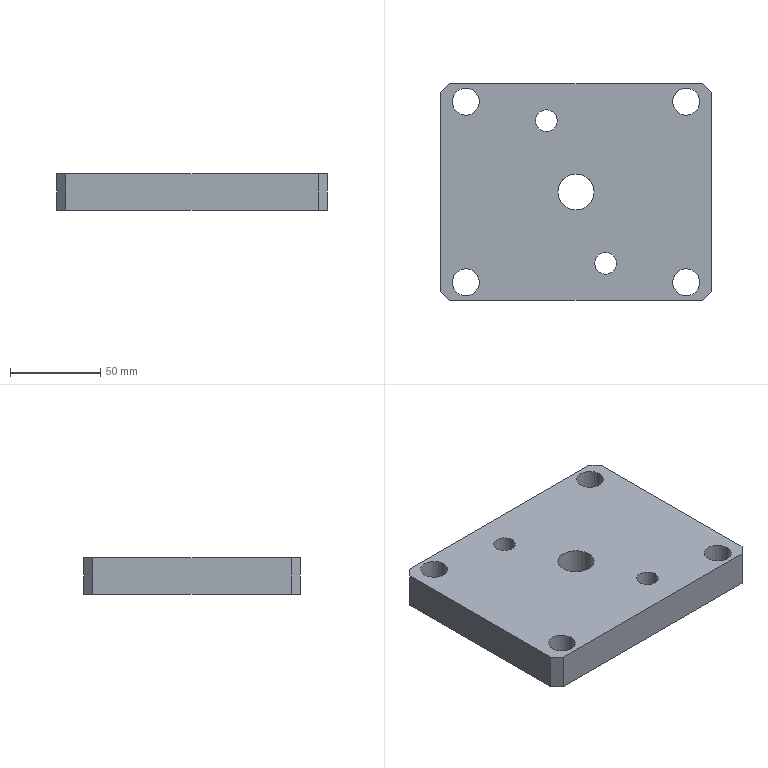Part | SolidWorks | features Cut 2, Extrusion 1, ICE 1 | 1 solid | 24 faces | box 150 x 120 x 20 mm | volume 334056 mm3 | cylinder 14 | plane 10 | commonest cylinder face diameters 15 x8 12 x4 20 x2
STEP:
#1=CARTESIAN_POINT('',(10.379,-39.542,20.));
#2=VERTEX_POINT('',#1);
#3=CARTESIAN_POINT('',(22.379,-39.542,20.));
#4=VERTEX_POINT('',#3);
#5=CARTESIAN_POINT('',(16.379,-39.542,20.));
#6=DIRECTION('',(0.,0.,1.));
#7=DIRECTION('',(-1.,0.,0.));
#8=AXIS2_PLACEMENT_3D('',#5,#6,#7);
#9=CIRCLE('',#8,6.);
#10=EDGE_CURVE('',#2,#4,#9,.T.);
#11=ORIENTED_EDGE('',*,*,#10,.T.);
#12=CARTESIAN_POINT('',(22.379,-39.542,0.));
#13=VERTEX_POINT('',#12);
#14=CARTESIAN_POINT('',(22.379,-39.542,36.971));
#15=DIRECTION('',(0.,0.,-1.));
#16=VECTOR('',#15,1000.);
#17=LINE('',#14,#16);
#18=EDGE_CURVE('',#4,#13,#17,.T.);
#19=ORIENTED_EDGE('',*,*,#18,.T.);
#20=CARTESIAN_POINT('',(10.379,-39.542,0.));
#21=VERTEX_POINT('',#20);
#22=CARTESIAN_POINT('',(16.379,-39.542,0.));
#23=DIRECTION('',(0.,0.,-1.));
#24=DIRECTION('',(-1.,0.,0.));
#25=AXIS2_PLACEMENT_3D('',#22,#23,#24);
#26=CIRCLE('',#25,6.);
#27=EDGE_CURVE('',#13,#21,#26,.T.);
#28=ORIENTED_EDGE('',*,*,#27,.T.);
#29=CARTESIAN_POINT('',(10.379,-39.542,36.971));
#30=DIRECTION('',(0.,0.,-1.));
#31=VECTOR('',#30,1000.);
#32=LINE('',#29,#31);
#33=EDGE_CURVE('',#2,#21,#32,.T.);
#34=ORIENTED_EDGE('',*,*,#33,.F.);
#35=EDGE_LOOP('',(#11,#19,#28,#34));
#36=FACE_OUTER_BOUND('',#35,.T.);
#37=CARTESIAN_POINT('',(16.379,-39.542,36.971));
#38=DIRECTION('',(0.,0.,-1.));
#39=DIRECTION('',(-1.,0.,0.));
#40=AXIS2_PLACEMENT_3D('',#37,#38,#39);
#41=CYLINDRICAL_SURFACE('',#40,6.);
#42=ADVANCED_FACE('',(#36),#41,.F.);
#43=CARTESIAN_POINT('',(-22.379,39.542,20.));
#44=VERTEX_POINT('',#43);
#45=CARTESIAN_POINT('',(-10.379,39.542,20.));
#46=VERTEX_POINT('',#45);
#47=CARTESIAN_POINT('',(-16.379,39.542,20.));
#48=DIRECTION('',(0.,0.,1.));
#49=DIRECTION('',(-1.,0.,0.));
#50=AXIS2_PLACEMENT_3D('',#47,#48,#49);
#51=CIRCLE('',#50,6.);
#52=EDGE_CURVE('',#44,#46,#51,.T.);
#53=ORIENTED_EDGE('',*,*,#52,.T.);
#54=CARTESIAN_POINT('',(-10.379,39.542,0.));
#55=VERTEX_POINT('',#54);
#56=CARTESIAN_POINT('',(-10.379,39.542,36.971));
#57=DIRECTION('',(0.,0.,-1.));
#58=VECTOR('',#57,1000.);
#59=LINE('',#56,#58);
#60=EDGE_CURVE('',#46,#55,#59,.T.);
#61=ORIENTED_EDGE('',*,*,#60,.T.);
#62=CARTESIAN_POINT('',(-22.379,39.542,0.));
#63=VERTEX_POINT('',#62);
#64=CARTESIAN_POINT('',(-16.379,39.542,0.));
#65=DIRECTION('',(0.,0.,-1.));
#66=DIRECTION('',(-1.,0.,0.));
#67=AXIS2_PLACEMENT_3D('',#64,#65,#66);
#68=CIRCLE('',#67,6.);
#69=EDGE_CURVE('',#55,#63,#68,.T.);
#70=ORIENTED_EDGE('',*,*,#69,.T.);
#71=CARTESIAN_POINT('',(-22.379,39.542,36.971));
#72=DIRECTION('',(0.,0.,-1.));
#73=VECTOR('',#72,1000.);
#74=LINE('',#71,#73);
#75=EDGE_CURVE('',#44,#63,#74,.T.);
#76=ORIENTED_EDGE('',*,*,#75,.F.);
#77=EDGE_LOOP('',(#53,#61,#70,#76));
#78=FACE_OUTER_BOUND('',#77,.T.);
#79=CARTESIAN_POINT('',(-16.379,39.542,36.971));
#80=DIRECTION('',(0.,0.,-1.));
#81=DIRECTION('',(-1.,0.,0.));
#82=AXIS2_PLACEMENT_3D('',#79,#80,#81);
#83=CYLINDRICAL_SURFACE('',#82,6.);
#84=ADVANCED_FACE('',(#78),#83,.F.);
#85=CARTESIAN_POINT('',(10.,0.,20.));
#86=VERTEX_POINT('',#85);
#87=CARTESIAN_POINT('',(-10.,0.,20.));
#88=VERTEX_POINT('',#87);
#89=CARTESIAN_POINT('',(0.,0.,20.));
#90=DIRECTION('',(0.,0.,-1.));
#91=DIRECTION('',(-1.,0.,0.));
#92=AXIS2_PLACEMENT_3D('',#89,#90,#91);
#93=CIRCLE('',#92,10.);
#94=EDGE_CURVE('',#86,#88,#93,.T.);
#95=ORIENTED_EDGE('',*,*,#94,.F.);
#96=CARTESIAN_POINT('',(10.,0.,0.));
#97=VERTEX_POINT('',#96);
#98=CARTESIAN_POINT('',(10.,0.,59.));
#99=DIRECTION('',(0.,0.,-1.));
#100=VECTOR('',#99,1000.);
#101=LINE('',#98,#100);
#102=EDGE_CURVE('',#86,#97,#101,.T.);
#103=ORIENTED_EDGE('',*,*,#102,.T.);
#104=CARTESIAN_POINT('',(-10.,0.,0.));
#105=VERTEX_POINT('',#104);
#106=CARTESIAN_POINT('',(0.,0.,0.));
#107=DIRECTION('',(0.,0.,-1.));
#108=DIRECTION('',(-1.,0.,0.));
#109=AXIS2_PLACEMENT_3D('',#106,#107,#108);
#110=CIRCLE('',#109,10.);
#111=EDGE_CURVE('',#97,#105,#110,.T.);
#112=ORIENTED_EDGE('',*,*,#111,.T.);
#113=CARTESIAN_POINT('',(-10.,0.,59.));
#114=DIRECTION('',(0.,0.,-1.));
#115=VECTOR('',#114,1000.);
#116=LINE('',#113,#115);
#117=EDGE_CURVE('',#88,#105,#116,.T.);
#118=ORIENTED_EDGE('',*,*,#117,.F.);
#119=EDGE_LOOP('',(#95,#103,#112,#118));
#120=FACE_OUTER_BOUND('',#119,.T.);
#121=CARTESIAN_POINT('',(0.,0.,59.));
#122=DIRECTION('',(0.,0.,-1.));
#123=DIRECTION('',(-1.,0.,0.));
#124=AXIS2_PLACEMENT_3D('',#121,#122,#123);
#125=CYLINDRICAL_SURFACE('',#124,10.);
#126=ADVANCED_FACE('',(#120),#125,.F.);
#127=CARTESIAN_POINT('',(-53.5,50.,20.));
#128=VERTEX_POINT('',#127);
#129=CARTESIAN_POINT('',(-68.5,50.,20.));
#130=VERTEX_POINT('',#129);
#131=CARTESIAN_POINT('',(-61.,50.,20.));
#132=DIRECTION('',(0.,0.,-1.));
#133=DIRECTION('',(1.,0.,0.));
#134=AXIS2_PLACEMENT_3D('',#131,#132,#133);
#135=CIRCLE('',#134,7.5);
#136=EDGE_CURVE('',#128,#130,#135,.T.);
#137=ORIENTED_EDGE('',*,*,#136,.F.);
#138=CARTESIAN_POINT('',(-53.5,50.,0.));
#139=VERTEX_POINT('',#138);
#140=CARTESIAN_POINT('',(-53.5,50.,20.));
#141=DIRECTION('',(0.,0.,-1.));
#142=VECTOR('',#141,1000.);
#143=LINE('',#140,#142);
#144=EDGE_CURVE('',#128,#139,#143,.T.);
#145=ORIENTED_EDGE('',*,*,#144,.T.);
#146=CARTESIAN_POINT('',(-68.5,50.,0.));
#147=VERTEX_POINT('',#146);
#148=CARTESIAN_POINT('',(-61.,50.,0.));
#149=DIRECTION('',(0.,0.,-1.));
#150=DIRECTION('',(-1.,0.,0.));
#151=AXIS2_PLACEMENT_3D('',#148,#149,#150);
#152=CIRCLE('',#151,7.5);
#153=EDGE_CURVE('',#139,#147,#152,.T.);
#154=ORIENTED_EDGE('',*,*,#153,.T.);
#155=CARTESIAN_POINT('',(-68.5,50.,20.));
#156=DIRECTION('',(0.,0.,-1.));
#157=VECTOR('',#156,1000.);
#158=LINE('',#155,#157);
#159=EDGE_CURVE('',#130,#147,#158,.T.);
#160=ORIENTED_EDGE('',*,*,#159,.F.);
#161=EDGE_LOOP('',(#137,#145,#154,#160));
#162=FACE_OUTER_BOUND('',#161,.T.);
#163=CARTESIAN_POINT('',(-61.,50.,20.));
#164=DIRECTION('',(0.,0.,-1.));
#165=DIRECTION('',(-1.,0.,0.));
#166=AXIS2_PLACEMENT_3D('',#163,#164,#165);
#167=CYLINDRICAL_SURFACE('',#166,7.5);
#168=ADVANCED_FACE('',(#162),#167,.F.);
#169=CARTESIAN_POINT('',(68.5,-50.,20.));
#170=VERTEX_POINT('',#169);
#171=CARTESIAN_POINT('',(53.5,-50.,20.));
#172=VERTEX_POINT('',#171);
#173=CARTESIAN_POINT('',(61.,-50.,20.));
#174=DIRECTION('',(0.,0.,-1.));
#175=DIRECTION('',(1.,0.,0.));
#176=AXIS2_PLACEMENT_3D('',#173,#174,#175);
#177=CIRCLE('',#176,7.5);
#178=EDGE_CURVE('',#170,#172,#177,.T.);
#179=ORIENTED_EDGE('',*,*,#178,.F.);
#180=CARTESIAN_POINT('',(68.5,-50.,0.));
#181=VERTEX_POINT('',#180);
#182=CARTESIAN_POINT('',(68.5,-50.,20.));
#183=DIRECTION('',(0.,0.,-1.));
#184=VECTOR('',#183,1000.);
#185=LINE('',#182,#184);
#186=EDGE_CURVE('',#170,#181,#185,.T.);
#187=ORIENTED_EDGE('',*,*,#186,.T.);
#188=CARTESIAN_POINT('',(53.5,-50.,0.));
#189=VERTEX_POINT('',#188);
#190=CARTESIAN_POINT('',(61.,-50.,0.));
#191=DIRECTION('',(0.,0.,-1.));
#192=DIRECTION('',(-1.,0.,0.));
#193=AXIS2_PLACEMENT_3D('',#190,#191,#192);
#194=CIRCLE('',#193,7.5);
#195=EDGE_CURVE('',#181,#189,#194,.T.);
#196=ORIENTED_EDGE('',*,*,#195,.T.);
#197=CARTESIAN_POINT('',(53.5,-50.,20.));
#198=DIRECTION('',(0.,0.,-1.));
#199=VECTOR('',#198,1000.);
#200=LINE('',#197,#199);
#201=EDGE_CURVE('',#172,#189,#200,.T.);
#202=ORIENTED_EDGE('',*,*,#201,.F.);
#203=EDGE_LOOP('',(#179,#187,#196,#202));
#204=FACE_OUTER_BOUND('',#203,.T.);
#205=CARTESIAN_POINT('',(61.,-50.,20.));
#206=DIRECTION('',(0.,0.,-1.));
#207=DIRECTION('',(-1.,0.,0.));
#208=AXIS2_PLACEMENT_3D('',#205,#206,#207);
#209=CYLINDRICAL_SURFACE('',#208,7.5);
#210=ADVANCED_FACE('',(#204),#209,.F.);
#211=CARTESIAN_POINT('',(68.5,50.,20.));
#212=VERTEX_POINT('',#211);
#213=CARTESIAN_POINT('',(53.5,50.,20.));
#214=VERTEX_POINT('',#213);
#215=CARTESIAN_POINT('',(61.,50.,20.));
#216=DIRECTION('',(0.,0.,-1.));
#217=DIRECTION('',(-1.,0.,0.));
#218=AXIS2_PLACEMENT_3D('',#215,#216,#217);
#219=CIRCLE('',#218,7.5);
#220=EDGE_CURVE('',#212,#214,#219,.T.);
#221=ORIENTED_EDGE('',*,*,#220,.F.);
#222=CARTESIAN_POINT('',(68.5,50.,0.));
#223=VERTEX_POINT('',#222);
#224=CARTESIAN_POINT('',(68.5,50.,20.));
#225=DIRECTION('',(0.,0.,-1.));
#226=VECTOR('',#225,1000.);
#227=LINE('',#224,#226);
#228=EDGE_CURVE('',#212,#223,#227,.T.);
#229=ORIENTED_EDGE('',*,*,#228,.T.);
#230=CARTESIAN_POINT('',(53.5,50.,0.));
#231=VERTEX_POINT('',#230);
#232=CARTESIAN_POINT('',(61.,50.,0.));
#233=DIRECTION('',(0.,0.,-1.));
#234=DIRECTION('',(-1.,0.,0.));
#235=AXIS2_PLACEMENT_3D('',#232,#233,#234);
#236=CIRCLE('',#235,7.5);
#237=EDGE_CURVE('',#223,#231,#236,.T.);
#238=ORIENTED_EDGE('',*,*,#237,.T.);
#239=CARTESIAN_POINT('',(53.5,50.,20.));
#240=DIRECTION('',(0.,0.,-1.));
#241=VECTOR('',#240,1000.);
#242=LINE('',#239,#241);
#243=EDGE_CURVE('',#214,#231,#242,.T.);
#244=ORIENTED_EDGE('',*,*,#243,.F.);
#245=EDGE_LOOP('',(#221,#229,#238,#244));
#246=FACE_OUTER_BOUND('',#245,.T.);
#247=CARTESIAN_POINT('',(61.,50.,20.));
#248=DIRECTION('',(0.,0.,-1.));
#249=DIRECTION('',(-1.,0.,0.));
#250=AXIS2_PLACEMENT_3D('',#247,#248,#249);
#251=CYLINDRICAL_SURFACE('',#250,7.5);
#252=ADVANCED_FACE('',(#246),#251,.F.);
#253=CARTESIAN_POINT('',(-53.5,-50.,20.));
#254=VERTEX_POINT('',#253);
#255=CARTESIAN_POINT('',(-68.5,-50.,20.));
#256=VERTEX_POINT('',#255);
#257=CARTESIAN_POINT('',(-61.,-50.,20.));
#258=DIRECTION('',(0.,0.,-1.));
#259=DIRECTION('',(-1.,0.,0.));
#260=AXIS2_PLACEMENT_3D('',#257,#258,#259);
#261=CIRCLE('',#260,7.5);
#262=EDGE_CURVE('',#254,#256,#261,.T.);
#263=ORIENTED_EDGE('',*,*,#262,.F.);
#264=CARTESIAN_POINT('',(-53.5,-50.,0.));
#265=VERTEX_POINT('',#264);
#266=CARTESIAN_POINT('',(-53.5,-50.,20.));
#267=DIRECTION('',(0.,0.,-1.));
#268=VECTOR('',#267,1000.);
#269=LINE('',#266,#268);
#270=EDGE_CURVE('',#254,#265,#269,.T.);
#271=ORIENTED_EDGE('',*,*,#270,.T.);
#272=CARTESIAN_POINT('',(-68.5,-50.,0.));
#273=VERTEX_POINT('',#272);
#274=CARTESIAN_POINT('',(-61.,-50.,0.));
#275=DIRECTION('',(0.,0.,-1.));
#276=DIRECTION('',(-1.,0.,0.));
#277=AXIS2_PLACEMENT_3D('',#274,#275,#276);
#278=CIRCLE('',#277,7.5);
#279=EDGE_CURVE('',#265,#273,#278,.T.);
#280=ORIENTED_EDGE('',*,*,#279,.T.);
#281=CARTESIAN_POINT('',(-68.5,-50.,20.));
#282=DIRECTION('',(0.,0.,-1.));
#283=VECTOR('',#282,1000.);
#284=LINE('',#281,#283);
#285=EDGE_CURVE('',#256,#273,#284,.T.);
#286=ORIENTED_EDGE('',*,*,#285,.F.);
#287=EDGE_LOOP('',(#263,#271,#280,#286));
#288=FACE_OUTER_BOUND('',#287,.T.);
#289=CARTESIAN_POINT('',(-61.,-50.,20.));
#290=DIRECTION('',(0.,0.,-1.));
#291=DIRECTION('',(-1.,0.,0.));
#292=AXIS2_PLACEMENT_3D('',#289,#290,#291);
#293=CYLINDRICAL_SURFACE('',#292,7.5);
#294=ADVANCED_FACE('',(#288),#293,.F.);
#295=CARTESIAN_POINT('',(-70.,-60.,0.));
#296=VERTEX_POINT('',#295);
#297=CARTESIAN_POINT('',(70.,-60.,0.));
#298=VERTEX_POINT('',#297);
#299=CARTESIAN_POINT('',(70.,-60.,0.));
#300=DIRECTION('',(1.,0.,0.));
#301=VECTOR('',#300,1000.);
#302=LINE('',#299,#301);
#303=EDGE_CURVE('',#296,#298,#302,.T.);
#304=ORIENTED_EDGE('',*,*,#303,.T.);
#305=CARTESIAN_POINT('',(70.,-60.,20.));
#306=VERTEX_POINT('',#305);
#307=CARTESIAN_POINT('',(70.,-60.,20.));
#308=DIRECTION('',(0.,0.,-1.));
#309=VECTOR('',#308,1000.);
#310=LINE('',#307,#309);
#311=EDGE_CURVE('',#306,#298,#310,.T.);
#312=ORIENTED_EDGE('',*,*,#311,.F.);
#313=CARTESIAN_POINT('',(-70.,-60.,20.));
#314=VERTEX_POINT('',#313);
#315=CARTESIAN_POINT('',(70.,-60.,20.));
#316=DIRECTION('',(1.,0.,0.));
#317=VECTOR('',#316,1000.);
#318=LINE('',#315,#317);
#319=EDGE_CURVE('',#314,#306,#318,.T.);
#320=ORIENTED_EDGE('',*,*,#319,.F.);
#321=CARTESIAN_POINT('',(-70.,-60.,20.));
#322=DIRECTION('',(0.,0.,-1.));
#323=VECTOR('',#322,1000.);
#324=LINE('',#321,#323);
#325=EDGE_CURVE('',#314,#296,#324,.T.);
#326=ORIENTED_EDGE('',*,*,#325,.T.);
#327=EDGE_LOOP('',(#304,#312,#320,#326));
#328=FACE_OUTER_BOUND('',#327,.T.);
#329=CARTESIAN_POINT('',(70.,-60.,20.));
#330=DIRECTION('',(0.,1.,0.));
#331=DIRECTION('',(-1.,0.,0.));
#332=AXIS2_PLACEMENT_3D('',#329,#330,#331);
#333=PLANE('',#332);
#334=ADVANCED_FACE('',(#328),#333,.F.);
#335=CARTESIAN_POINT('',(75.,-55.,0.));
#336=VERTEX_POINT('',#335);
#337=CARTESIAN_POINT('',(75.,-55.,0.));
#338=DIRECTION('',(0.7071,0.7071,0.));
#339=VECTOR('',#338,1000.);
#340=LINE('',#337,#339);
#341=EDGE_CURVE('',#298,#336,#340,.T.);
#342=ORIENTED_EDGE('',*,*,#341,.T.);
#343=CARTESIAN_POINT('',(75.,-55.,20.));
#344=VERTEX_POINT('',#343);
#345=CARTESIAN_POINT('',(75.,-55.,20.));
#346=DIRECTION('',(0.,0.,-1.));
#347=VECTOR('',#346,1000.);
#348=LINE('',#345,#347);
#349=EDGE_CURVE('',#344,#336,#348,.T.);
#350=ORIENTED_EDGE('',*,*,#349,.F.);
#351=CARTESIAN_POINT('',(75.,-55.,20.));
#352=DIRECTION('',(0.7071,0.7071,0.));
#353=VECTOR('',#352,1000.);
#354=LINE('',#351,#353);
#355=EDGE_CURVE('',#306,#344,#354,.T.);
#356=ORIENTED_EDGE('',*,*,#355,.F.);
#357=ORIENTED_EDGE('',*,*,#311,.T.);
#358=EDGE_LOOP('',(#342,#350,#356,#357));
#359=FACE_OUTER_BOUND('',#358,.T.);
#360=CARTESIAN_POINT('',(75.,-55.,20.));
#361=DIRECTION('',(-0.7071,0.7071,0.));
#362=DIRECTION('',(-0.7071,-0.7071,0.));
#363=AXIS2_PLACEMENT_3D('',#360,#361,#362);
#364=PLANE('',#363);
#365=ADVANCED_FACE('',(#359),#364,.F.);
#366=CARTESIAN_POINT('',(75.,55.,0.));
#367=VERTEX_POINT('',#366);
#368=CARTESIAN_POINT('',(75.,-55.,0.));
#369=DIRECTION('',(0.,1.,0.));
#370=VECTOR('',#369,1000.);
#371=LINE('',#368,#370);
#372=EDGE_CURVE('',#336,#367,#371,.T.);
#373=ORIENTED_EDGE('',*,*,#372,.T.);
#374=CARTESIAN_POINT('',(75.,55.,20.));
#375=VERTEX_POINT('',#374);
#376=CARTESIAN_POINT('',(75.,55.,20.));
#377=DIRECTION('',(0.,0.,-1.));
#378=VECTOR('',#377,1000.);
#379=LINE('',#376,#378);
#380=EDGE_CURVE('',#375,#367,#379,.T.);
#381=ORIENTED_EDGE('',*,*,#380,.F.);
#382=CARTESIAN_POINT('',(75.,-55.,20.));
#383=DIRECTION('',(0.,1.,0.));
#384=VECTOR('',#383,1000.);
#385=LINE('',#382,#384);
#386=EDGE_CURVE('',#344,#375,#385,.T.);
#387=ORIENTED_EDGE('',*,*,#386,.F.);
#388=ORIENTED_EDGE('',*,*,#349,.T.);
#389=EDGE_LOOP('',(#373,#381,#387,#388));
#390=FACE_OUTER_BOUND('',#389,.T.);
#391=CARTESIAN_POINT('',(75.,-55.,20.));
#392=DIRECTION('',(-1.,0.,0.));
#393=DIRECTION('',(0.,0.,1.));
#394=AXIS2_PLACEMENT_3D('',#391,#392,#393);
#395=PLANE('',#394);
#396=ADVANCED_FACE('',(#390),#395,.F.);
#397=CARTESIAN_POINT('',(70.,60.,0.));
#398=VERTEX_POINT('',#397);
#399=CARTESIAN_POINT('',(75.,55.,0.));
#400=DIRECTION('',(-0.7071,0.7071,0.));
#401=VECTOR('',#400,1000.);
#402=LINE('',#399,#401);
#403=EDGE_CURVE('',#367,#398,#402,.T.);
#404=ORIENTED_EDGE('',*,*,#403,.T.);
#405=CARTESIAN_POINT('',(70.,60.,20.));
#406=VERTEX_POINT('',#405);
#407=CARTESIAN_POINT('',(70.,60.,20.));
#408=DIRECTION('',(0.,0.,-1.));
#409=VECTOR('',#408,1000.);
#410=LINE('',#407,#409);
#411=EDGE_CURVE('',#406,#398,#410,.T.);
#412=ORIENTED_EDGE('',*,*,#411,.F.);
#413=CARTESIAN_POINT('',(75.,55.,20.));
#414=DIRECTION('',(-0.7071,0.7071,0.));
#415=VECTOR('',#414,1000.);
#416=LINE('',#413,#415);
#417=EDGE_CURVE('',#375,#406,#416,.T.);
#418=ORIENTED_EDGE('',*,*,#417,.F.);
#419=ORIENTED_EDGE('',*,*,#380,.T.);
#420=EDGE_LOOP('',(#404,#412,#418,#419));
#421=FACE_OUTER_BOUND('',#420,.T.);
#422=CARTESIAN_POINT('',(75.,55.,20.));
#423=DIRECTION('',(-0.7071,-0.7071,0.));
#424=DIRECTION('',(0.7071,-0.7071,0.));
#425=AXIS2_PLACEMENT_3D('',#422,#423,#424);
#426=PLANE('',#425);
#427=ADVANCED_FACE('',(#421),#426,.F.);
#428=CARTESIAN_POINT('',(-70.,60.,0.));
#429=VERTEX_POINT('',#428);
#430=CARTESIAN_POINT('',(70.,60.,0.));
#431=DIRECTION('',(-1.,0.,0.));
#432=VECTOR('',#431,1000.);
#433=LINE('',#430,#432);
#434=EDGE_CURVE('',#398,#429,#433,.T.);
#435=ORIENTED_EDGE('',*,*,#434,.T.);
#436=CARTESIAN_POINT('',(-70.,60.,20.));
#437=VERTEX_POINT('',#436);
#438=CARTESIAN_POINT('',(-70.,60.,20.));
#439=DIRECTION('',(0.,0.,-1.));
#440=VECTOR('',#439,1000.);
#441=LINE('',#438,#440);
#442=EDGE_CURVE('',#437,#429,#441,.T.);
#443=ORIENTED_EDGE('',*,*,#442,.F.);
#444=CARTESIAN_POINT('',(70.,60.,20.));
#445=DIRECTION('',(-1.,0.,0.));
#446=VECTOR('',#445,1000.);
#447=LINE('',#444,#446);
#448=EDGE_CURVE('',#406,#437,#447,.T.);
#449=ORIENTED_EDGE('',*,*,#448,.F.);
#450=ORIENTED_EDGE('',*,*,#411,.T.);
#451=EDGE_LOOP('',(#435,#443,#449,#450));
#452=FACE_OUTER_BOUND('',#451,.T.);
#453=CARTESIAN_POINT('',(70.,60.,20.));
#454=DIRECTION('',(0.,-1.,0.));
#455=DIRECTION('',(1.,0.,0.));
#456=AXIS2_PLACEMENT_3D('',#453,#454,#455);
#457=PLANE('',#456);
#458=ADVANCED_FACE('',(#452),#457,.F.);
#459=CARTESIAN_POINT('',(-75.,55.,0.));
#460=VERTEX_POINT('',#459);
#461=CARTESIAN_POINT('',(-75.,55.,0.));
#462=DIRECTION('',(-0.7071,-0.7071,0.));
#463=VECTOR('',#462,1000.);
#464=LINE('',#461,#463);
#465=EDGE_CURVE('',#429,#460,#464,.T.);
#466=ORIENTED_EDGE('',*,*,#465,.T.);
#467=CARTESIAN_POINT('',(-75.,55.,20.));
#468=VERTEX_POINT('',#467);
#469=CARTESIAN_POINT('',(-75.,55.,20.));
#470=DIRECTION('',(0.,0.,-1.));
#471=VECTOR('',#470,1000.);
#472=LINE('',#469,#471);
#473=EDGE_CURVE('',#468,#460,#472,.T.);
#474=ORIENTED_EDGE('',*,*,#473,.F.);
#475=CARTESIAN_POINT('',(-75.,55.,20.));
#476=DIRECTION('',(-0.7071,-0.7071,0.));
#477=VECTOR('',#476,1000.);
#478=LINE('',#475,#477);
#479=EDGE_CURVE('',#437,#468,#478,.T.);
#480=ORIENTED_EDGE('',*,*,#479,.F.);
#481=ORIENTED_EDGE('',*,*,#442,.T.);
#482=EDGE_LOOP('',(#466,#474,#480,#481));
#483=FACE_OUTER_BOUND('',#482,.T.);
#484=CARTESIAN_POINT('',(-75.,55.,20.));
#485=DIRECTION('',(0.7071,-0.7071,0.));
#486=DIRECTION('',(0.7071,0.7071,0.));
#487=AXIS2_PLACEMENT_3D('',#484,#485,#486);
#488=PLANE('',#487);
#489=ADVANCED_FACE('',(#483),#488,.F.);
#490=CARTESIAN_POINT('',(-75.,-55.,0.));
#491=VERTEX_POINT('',#490);
#492=CARTESIAN_POINT('',(-75.,-55.,0.));
#493=DIRECTION('',(0.,-1.,0.));
#494=VECTOR('',#493,1000.);
#495=LINE('',#492,#494);
#496=EDGE_CURVE('',#460,#491,#495,.T.);
#497=ORIENTED_EDGE('',*,*,#496,.T.);
#498=CARTESIAN_POINT('',(-75.,-55.,20.));
#499=VERTEX_POINT('',#498);
#500=CARTESIAN_POINT('',(-75.,-55.,20.));
#501=DIRECTION('',(0.,0.,-1.));
#502=VECTOR('',#501,1000.);
#503=LINE('',#500,#502);
#504=EDGE_CURVE('',#499,#491,#503,.T.);
#505=ORIENTED_EDGE('',*,*,#504,.F.);
#506=CARTESIAN_POINT('',(-75.,-55.,20.));
#507=DIRECTION('',(0.,-1.,0.));
#508=VECTOR('',#507,1000.);
#509=LINE('',#506,#508);
#510=EDGE_CURVE('',#468,#499,#509,.T.);
#511=ORIENTED_EDGE('',*,*,#510,.F.);
#512=ORIENTED_EDGE('',*,*,#473,.T.);
#513=EDGE_LOOP('',(#497,#505,#511,#512));
#514=FACE_OUTER_BOUND('',#513,.T.);
#515=CARTESIAN_POINT('',(-75.,-55.,20.));
#516=DIRECTION('',(1.,0.,0.));
#517=DIRECTION('',(0.,0.,-1.));
#518=AXIS2_PLACEMENT_3D('',#515,#516,#517);
#519=PLANE('',#518);
#520=ADVANCED_FACE('',(#514),#519,.F.);
#521=CARTESIAN_POINT('',(-70.,-60.,0.));
#522=DIRECTION('',(0.7071,-0.7071,0.));
#523=VECTOR('',#522,1000.);
#524=LINE('',#521,#523);
#525=EDGE_CURVE('',#491,#296,#524,.T.);
#526=ORIENTED_EDGE('',*,*,#525,.T.);
#527=ORIENTED_EDGE('',*,*,#325,.F.);
#528=CARTESIAN_POINT('',(-70.,-60.,20.));
#529=DIRECTION('',(0.7071,-0.7071,0.));
#530=VECTOR('',#529,1000.);
#531=LINE('',#528,#530);
#532=EDGE_CURVE('',#499,#314,#531,.T.);
#533=ORIENTED_EDGE('',*,*,#532,.F.);
#534=ORIENTED_EDGE('',*,*,#504,.T.);
#535=EDGE_LOOP('',(#526,#527,#533,#534));
#536=FACE_OUTER_BOUND('',#535,.T.);
#537=CARTESIAN_POINT('',(-70.,-60.,20.));
#538=DIRECTION('',(0.7071,0.7071,0.));
#539=DIRECTION('',(-0.7071,0.7071,0.));
#540=AXIS2_PLACEMENT_3D('',#537,#538,#539);
#541=PLANE('',#540);
#542=ADVANCED_FACE('',(#536),#541,.F.);
#543=ORIENTED_EDGE('',*,*,#10,.F.);
#544=CARTESIAN_POINT('',(16.379,-39.542,20.));
#545=DIRECTION('',(0.,0.,1.));
#546=DIRECTION('',(-1.,0.,0.));
#547=AXIS2_PLACEMENT_3D('',#544,#545,#546);
#548=CIRCLE('',#547,6.);
#549=EDGE_CURVE('',#4,#2,#548,.T.);
#550=ORIENTED_EDGE('',*,*,#549,.F.);
#551=EDGE_LOOP('',(#543,#550));
#552=FACE_BOUND('',#551,.T.);
#553=ORIENTED_EDGE('',*,*,#52,.F.);
#554=CARTESIAN_POINT('',(-16.379,39.542,20.));
#555=DIRECTION('',(0.,0.,1.));
#556=DIRECTION('',(-1.,0.,0.));
#557=AXIS2_PLACEMENT_3D('',#554,#555,#556);
#558=CIRCLE('',#557,6.);
#559=EDGE_CURVE('',#46,#44,#558,.T.);
#560=ORIENTED_EDGE('',*,*,#559,.F.);
#561=EDGE_LOOP('',(#553,#560));
#562=FACE_BOUND('',#561,.T.);
#563=CARTESIAN_POINT('',(0.,0.,20.));
#564=DIRECTION('',(0.,0.,-1.));
#565=DIRECTION('',(-1.,0.,0.));
#566=AXIS2_PLACEMENT_3D('',#563,#564,#565);
#567=CIRCLE('',#566,10.);
#568=EDGE_CURVE('',#88,#86,#567,.T.);
#569=ORIENTED_EDGE('',*,*,#568,.T.);
#570=ORIENTED_EDGE('',*,*,#94,.T.);
#571=EDGE_LOOP('',(#569,#570));
#572=FACE_BOUND('',#571,.T.);
#573=CARTESIAN_POINT('',(-61.,50.,20.));
#574=DIRECTION('',(0.,0.,-1.));
#575=DIRECTION('',(1.,0.,0.));
#576=AXIS2_PLACEMENT_3D('',#573,#574,#575);
#577=CIRCLE('',#576,7.5);
#578=EDGE_CURVE('',#130,#128,#577,.T.);
#579=ORIENTED_EDGE('',*,*,#578,.T.);
#580=ORIENTED_EDGE('',*,*,#136,.T.);
#581=EDGE_LOOP('',(#579,#580));
#582=FACE_BOUND('',#581,.T.);
#583=CARTESIAN_POINT('',(61.,-50.,20.));
#584=DIRECTION('',(0.,0.,-1.));
#585=DIRECTION('',(1.,0.,0.));
#586=AXIS2_PLACEMENT_3D('',#583,#584,#585);
#587=CIRCLE('',#586,7.5);
#588=EDGE_CURVE('',#172,#170,#587,.T.);
#589=ORIENTED_EDGE('',*,*,#588,.T.);
#590=ORIENTED_EDGE('',*,*,#178,.T.);
#591=EDGE_LOOP('',(#589,#590));
#592=FACE_BOUND('',#591,.T.);
#593=CARTESIAN_POINT('',(61.,50.,20.));
#594=DIRECTION('',(0.,0.,-1.));
#595=DIRECTION('',(-1.,0.,0.));
#596=AXIS2_PLACEMENT_3D('',#593,#594,#595);
#597=CIRCLE('',#596,7.5);
#598=EDGE_CURVE('',#214,#212,#597,.T.);
#599=ORIENTED_EDGE('',*,*,#598,.T.);
#600=ORIENTED_EDGE('',*,*,#220,.T.);
#601=EDGE_LOOP('',(#599,#600));
#602=FACE_BOUND('',#601,.T.);
#603=CARTESIAN_POINT('',(-61.,-50.,20.));
#604=DIRECTION('',(0.,0.,-1.));
#605=DIRECTION('',(-1.,0.,0.));
#606=AXIS2_PLACEMENT_3D('',#603,#604,#605);
#607=CIRCLE('',#606,7.5);
#608=EDGE_CURVE('',#256,#254,#607,.T.);
#609=ORIENTED_EDGE('',*,*,#608,.T.);
#610=ORIENTED_EDGE('',*,*,#262,.T.);
#611=EDGE_LOOP('',(#609,#610));
#612=FACE_BOUND('',#611,.T.);
#613=ORIENTED_EDGE('',*,*,#319,.T.);
#614=ORIENTED_EDGE('',*,*,#355,.T.);
#615=ORIENTED_EDGE('',*,*,#386,.T.);
#616=ORIENTED_EDGE('',*,*,#417,.T.);
#617=ORIENTED_EDGE('',*,*,#448,.T.);
#618=ORIENTED_EDGE('',*,*,#479,.T.);
#619=ORIENTED_EDGE('',*,*,#510,.T.);
#620=ORIENTED_EDGE('',*,*,#532,.T.);
#621=EDGE_LOOP('',(#613,#614,#615,#616,#617,#618,#619,#620));
#622=FACE_OUTER_BOUND('',#621,.T.);
#623=CARTESIAN_POINT('',(0.,0.,20.));
#624=DIRECTION('',(0.,0.,-1.));
#625=DIRECTION('',(-1.,0.,0.));
#626=AXIS2_PLACEMENT_3D('',#623,#624,#625);
#627=PLANE('',#626);
#628=ADVANCED_FACE('',(#552,#562,#572,#582,#592,#602,#612,#622),#627,.F.);
#629=CARTESIAN_POINT('',(16.379,-39.542,0.));
#630=DIRECTION('',(0.,0.,-1.));
#631=DIRECTION('',(-1.,0.,0.));
#632=AXIS2_PLACEMENT_3D('',#629,#630,#631);
#633=CIRCLE('',#632,6.);
#634=EDGE_CURVE('',#21,#13,#633,.T.);
#635=ORIENTED_EDGE('',*,*,#634,.F.);
#636=ORIENTED_EDGE('',*,*,#27,.F.);
#637=EDGE_LOOP('',(#635,#636));
#638=FACE_BOUND('',#637,.T.);
#639=CARTESIAN_POINT('',(-16.379,39.542,0.));
#640=DIRECTION('',(0.,0.,-1.));
#641=DIRECTION('',(-1.,0.,0.));
#642=AXIS2_PLACEMENT_3D('',#639,#640,#641);
#643=CIRCLE('',#642,6.);
#644=EDGE_CURVE('',#63,#55,#643,.T.);
#645=ORIENTED_EDGE('',*,*,#644,.F.);
#646=ORIENTED_EDGE('',*,*,#69,.F.);
#647=EDGE_LOOP('',(#645,#646));
#648=FACE_BOUND('',#647,.T.);
#649=CARTESIAN_POINT('',(0.,0.,0.));
#650=DIRECTION('',(0.,0.,-1.));
#651=DIRECTION('',(-1.,0.,0.));
#652=AXIS2_PLACEMENT_3D('',#649,#650,#651);
#653=CIRCLE('',#652,10.);
#654=EDGE_CURVE('',#105,#97,#653,.T.);
#655=ORIENTED_EDGE('',*,*,#654,.F.);
#656=ORIENTED_EDGE('',*,*,#111,.F.);
#657=EDGE_LOOP('',(#655,#656));
#658=FACE_BOUND('',#657,.T.);
#659=CARTESIAN_POINT('',(-61.,50.,0.));
#660=DIRECTION('',(0.,0.,-1.));
#661=DIRECTION('',(-1.,0.,0.));
#662=AXIS2_PLACEMENT_3D('',#659,#660,#661);
#663=CIRCLE('',#662,7.5);
#664=EDGE_CURVE('',#147,#139,#663,.T.);
#665=ORIENTED_EDGE('',*,*,#664,.F.);
#666=ORIENTED_EDGE('',*,*,#153,.F.);
#667=EDGE_LOOP('',(#665,#666));
#668=FACE_BOUND('',#667,.T.);
#669=CARTESIAN_POINT('',(61.,-50.,0.));
#670=DIRECTION('',(0.,0.,-1.));
#671=DIRECTION('',(-1.,0.,0.));
#672=AXIS2_PLACEMENT_3D('',#669,#670,#671);
#673=CIRCLE('',#672,7.5);
#674=EDGE_CURVE('',#189,#181,#673,.T.);
#675=ORIENTED_EDGE('',*,*,#674,.F.);
#676=ORIENTED_EDGE('',*,*,#195,.F.);
#677=EDGE_LOOP('',(#675,#676));
#678=FACE_BOUND('',#677,.T.);
#679=CARTESIAN_POINT('',(61.,50.,0.));
#680=DIRECTION('',(0.,0.,-1.));
#681=DIRECTION('',(-1.,0.,0.));
#682=AXIS2_PLACEMENT_3D('',#679,#680,#681);
#683=CIRCLE('',#682,7.5);
#684=EDGE_CURVE('',#231,#223,#683,.T.);
#685=ORIENTED_EDGE('',*,*,#684,.F.);
#686=ORIENTED_EDGE('',*,*,#237,.F.);
#687=EDGE_LOOP('',(#685,#686));
#688=FACE_BOUND('',#687,.T.);
#689=CARTESIAN_POINT('',(-61.,-50.,0.));
#690=DIRECTION('',(0.,0.,-1.));
#691=DIRECTION('',(-1.,0.,0.));
#692=AXIS2_PLACEMENT_3D('',#689,#690,#691);
#693=CIRCLE('',#692,7.5);
#694=EDGE_CURVE('',#273,#265,#693,.T.);
#695=ORIENTED_EDGE('',*,*,#694,.F.);
#696=ORIENTED_EDGE('',*,*,#279,.F.);
#697=EDGE_LOOP('',(#695,#696));
#698=FACE_BOUND('',#697,.T.);
#699=ORIENTED_EDGE('',*,*,#303,.F.);
#700=ORIENTED_EDGE('',*,*,#525,.F.);
#701=ORIENTED_EDGE('',*,*,#496,.F.);
#702=ORIENTED_EDGE('',*,*,#465,.F.);
#703=ORIENTED_EDGE('',*,*,#434,.F.);
#704=ORIENTED_EDGE('',*,*,#403,.F.);
#705=ORIENTED_EDGE('',*,*,#372,.F.);
#706=ORIENTED_EDGE('',*,*,#341,.F.);
#707=EDGE_LOOP('',(#699,#700,#701,#702,#703,#704,#705,#706));
#708=FACE_OUTER_BOUND('',#707,.T.);
#709=CARTESIAN_POINT('',(0.,0.,0.));
#710=DIRECTION('',(0.,0.,-1.));
#711=DIRECTION('',(-1.,0.,0.));
#712=AXIS2_PLACEMENT_3D('',#709,#710,#711);
#713=PLANE('',#712);
#714=ADVANCED_FACE('',(#638,#648,#658,#668,#678,#688,#698,#708),#713,.T.);
#715=ORIENTED_EDGE('',*,*,#270,.F.);
#716=ORIENTED_EDGE('',*,*,#608,.F.);
#717=ORIENTED_EDGE('',*,*,#285,.T.);
#718=ORIENTED_EDGE('',*,*,#694,.T.);
#719=EDGE_LOOP('',(#715,#716,#717,#718));
#720=FACE_OUTER_BOUND('',#719,.T.);
#721=CARTESIAN_POINT('',(-61.,-50.,20.));
#722=DIRECTION('',(0.,0.,-1.));
#723=DIRECTION('',(-1.,0.,0.));
#724=AXIS2_PLACEMENT_3D('',#721,#722,#723);
#725=CYLINDRICAL_SURFACE('',#724,7.5);
#726=ADVANCED_FACE('',(#720),#725,.F.);
#727=ORIENTED_EDGE('',*,*,#228,.F.);
#728=ORIENTED_EDGE('',*,*,#598,.F.);
#729=ORIENTED_EDGE('',*,*,#243,.T.);
#730=ORIENTED_EDGE('',*,*,#684,.T.);
#731=EDGE_LOOP('',(#727,#728,#729,#730));
#732=FACE_OUTER_BOUND('',#731,.T.);
#733=CARTESIAN_POINT('',(61.,50.,20.));
#734=DIRECTION('',(0.,0.,-1.));
#735=DIRECTION('',(-1.,0.,0.));
#736=AXIS2_PLACEMENT_3D('',#733,#734,#735);
#737=CYLINDRICAL_SURFACE('',#736,7.5);
#738=ADVANCED_FACE('',(#732),#737,.F.);
#739=ORIENTED_EDGE('',*,*,#186,.F.);
#740=ORIENTED_EDGE('',*,*,#588,.F.);
#741=ORIENTED_EDGE('',*,*,#201,.T.);
#742=ORIENTED_EDGE('',*,*,#674,.T.);
#743=EDGE_LOOP('',(#739,#740,#741,#742));
#744=FACE_OUTER_BOUND('',#743,.T.);
#745=CARTESIAN_POINT('',(61.,-50.,20.));
#746=DIRECTION('',(0.,0.,-1.));
#747=DIRECTION('',(-1.,0.,0.));
#748=AXIS2_PLACEMENT_3D('',#745,#746,#747);
#749=CYLINDRICAL_SURFACE('',#748,7.5);
#750=ADVANCED_FACE('',(#744),#749,.F.);
#751=ORIENTED_EDGE('',*,*,#144,.F.);
#752=ORIENTED_EDGE('',*,*,#578,.F.);
#753=ORIENTED_EDGE('',*,*,#159,.T.);
#754=ORIENTED_EDGE('',*,*,#664,.T.);
#755=EDGE_LOOP('',(#751,#752,#753,#754));
#756=FACE_OUTER_BOUND('',#755,.T.);
#757=CARTESIAN_POINT('',(-61.,50.,20.));
#758=DIRECTION('',(0.,0.,-1.));
#759=DIRECTION('',(-1.,0.,0.));
#760=AXIS2_PLACEMENT_3D('',#757,#758,#759);
#761=CYLINDRICAL_SURFACE('',#760,7.5);
#762=ADVANCED_FACE('',(#756),#761,.F.);
#763=ORIENTED_EDGE('',*,*,#102,.F.);
#764=ORIENTED_EDGE('',*,*,#568,.F.);
#765=ORIENTED_EDGE('',*,*,#117,.T.);
#766=ORIENTED_EDGE('',*,*,#654,.T.);
#767=EDGE_LOOP('',(#763,#764,#765,#766));
#768=FACE_OUTER_BOUND('',#767,.T.);
#769=CARTESIAN_POINT('',(0.,0.,59.));
#770=DIRECTION('',(0.,0.,-1.));
#771=DIRECTION('',(-1.,0.,0.));
#772=AXIS2_PLACEMENT_3D('',#769,#770,#771);
#773=CYLINDRICAL_SURFACE('',#772,10.);
#774=ADVANCED_FACE('',(#768),#773,.F.);
#775=ORIENTED_EDGE('',*,*,#60,.F.);
#776=ORIENTED_EDGE('',*,*,#559,.T.);
#777=ORIENTED_EDGE('',*,*,#75,.T.);
#778=ORIENTED_EDGE('',*,*,#644,.T.);
#779=EDGE_LOOP('',(#775,#776,#777,#778));
#780=FACE_OUTER_BOUND('',#779,.T.);
#781=CARTESIAN_POINT('',(-16.379,39.542,36.971));
#782=DIRECTION('',(0.,0.,-1.));
#783=DIRECTION('',(-1.,0.,0.));
#784=AXIS2_PLACEMENT_3D('',#781,#782,#783);
#785=CYLINDRICAL_SURFACE('',#784,6.);
#786=ADVANCED_FACE('',(#780),#785,.F.);
#787=ORIENTED_EDGE('',*,*,#18,.F.);
#788=ORIENTED_EDGE('',*,*,#549,.T.);
#789=ORIENTED_EDGE('',*,*,#33,.T.);
#790=ORIENTED_EDGE('',*,*,#634,.T.);
#791=EDGE_LOOP('',(#787,#788,#789,#790));
#792=FACE_OUTER_BOUND('',#791,.T.);
#793=CARTESIAN_POINT('',(16.379,-39.542,36.971));
#794=DIRECTION('',(0.,0.,-1.));
#795=DIRECTION('',(-1.,0.,0.));
#796=AXIS2_PLACEMENT_3D('',#793,#794,#795);
#797=CYLINDRICAL_SURFACE('',#796,6.);
#798=ADVANCED_FACE('',(#792),#797,.F.);
#799=CLOSED_SHELL('',(#42,#84,#126,#168,#210,#252,#294,#334,#365,#396,#427,#458,#489,#520,#542,#628,#714,#726,#738,#750,#762,#774,#786,#798));
#800=MANIFOLD_SOLID_BREP('',#799);
#801=CARTESIAN_POINT('',(0.,0.,0.));
#802=DIRECTION('',(0.,0.,1.));
#803=DIRECTION('',(1.,0.,0.));
#804=AXIS2_PLACEMENT_3D('',#801,#802,#803);
#805=(LENGTH_UNIT()NAMED_UNIT(*)SI_UNIT(.MILLI.,.METRE.));
#806=UNCERTAINTY_MEASURE_WITH_UNIT(LENGTH_MEASURE(0.00001),#805,'','');
#807=(NAMED_UNIT(*)PLANE_ANGLE_UNIT()SI_UNIT($,.RADIAN.));
#808=(NAMED_UNIT(*)SI_UNIT($,.STERADIAN.)SOLID_ANGLE_UNIT());
#809=(GEOMETRIC_REPRESENTATION_CONTEXT(3)GLOBAL_UNCERTAINTY_ASSIGNED_CONTEXT((#806))GLOBAL_UNIT_ASSIGNED_CONTEXT((#805,#807,#808))REPRESENTATION_CONTEXT('',''));
#810=ADVANCED_BREP_SHAPE_REPRESENTATION('',(#800,#804),#809);